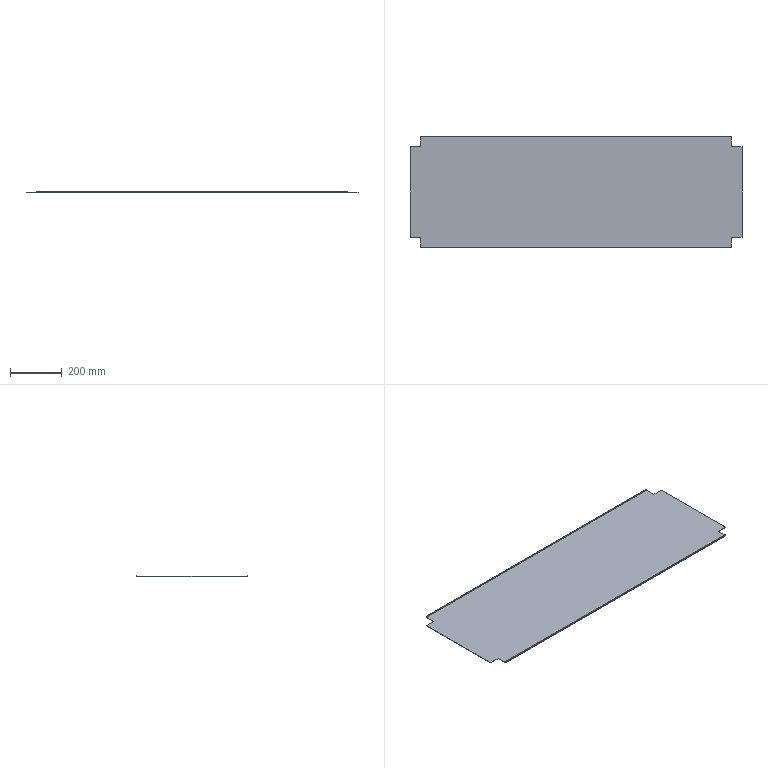Part | SolidWorks | features Extrusion 1, ICE 1 | 1 solid | 18 faces | box 1280 x 430 x 6.5 mm | volume 834000 mm3 | plane 18
STEP:
#1=CARTESIAN_POINT('',(40.,40.,1.5));
#2=VERTEX_POINT('',#1);
#3=CARTESIAN_POINT('',(40.,1.5,1.5));
#4=VERTEX_POINT('',#3);
#5=CARTESIAN_POINT('',(40.,0.,1.5));
#6=DIRECTION('',(0.,-1.,0.));
#7=VECTOR('',#6,1000.);
#8=LINE('',#5,#7);
#9=EDGE_CURVE('',#2,#4,#8,.T.);
#10=ORIENTED_EDGE('',*,*,#9,.T.);
#11=CARTESIAN_POINT('',(1240.,1.5,1.5));
#12=VERTEX_POINT('',#11);
#13=CARTESIAN_POINT('',(40.,1.5,1.5));
#14=DIRECTION('',(-1.,0.,0.));
#15=VECTOR('',#14,1000.);
#16=LINE('',#13,#15);
#17=EDGE_CURVE('',#12,#4,#16,.T.);
#18=ORIENTED_EDGE('',*,*,#17,.F.);
#19=CARTESIAN_POINT('',(1240.,40.,1.5));
#20=VERTEX_POINT('',#19);
#21=CARTESIAN_POINT('',(1240.,0.,1.5));
#22=DIRECTION('',(0.,1.,0.));
#23=VECTOR('',#22,1000.);
#24=LINE('',#21,#23);
#25=EDGE_CURVE('',#12,#20,#24,.T.);
#26=ORIENTED_EDGE('',*,*,#25,.T.);
#27=CARTESIAN_POINT('',(1280.,40.,1.5));
#28=VERTEX_POINT('',#27);
#29=CARTESIAN_POINT('',(1280.,40.,1.5));
#30=DIRECTION('',(1.,0.,0.));
#31=VECTOR('',#30,1000.);
#32=LINE('',#29,#31);
#33=EDGE_CURVE('',#20,#28,#32,.T.);
#34=ORIENTED_EDGE('',*,*,#33,.T.);
#35=CARTESIAN_POINT('',(1280.,390.,1.5));
#36=VERTEX_POINT('',#35);
#37=CARTESIAN_POINT('',(1280.,40.,1.5));
#38=DIRECTION('',(0.,1.,0.));
#39=VECTOR('',#38,1000.);
#40=LINE('',#37,#39);
#41=EDGE_CURVE('',#28,#36,#40,.T.);
#42=ORIENTED_EDGE('',*,*,#41,.T.);
#43=CARTESIAN_POINT('',(1240.,390.,1.5));
#44=VERTEX_POINT('',#43);
#45=CARTESIAN_POINT('',(1280.,390.,1.5));
#46=DIRECTION('',(-1.,0.,0.));
#47=VECTOR('',#46,1000.);
#48=LINE('',#45,#47);
#49=EDGE_CURVE('',#36,#44,#48,.T.);
#50=ORIENTED_EDGE('',*,*,#49,.T.);
#51=CARTESIAN_POINT('',(1240.,428.5,1.5));
#52=VERTEX_POINT('',#51);
#53=CARTESIAN_POINT('',(1240.,430.,1.5));
#54=DIRECTION('',(0.,1.,0.));
#55=VECTOR('',#54,1000.);
#56=LINE('',#53,#55);
#57=EDGE_CURVE('',#44,#52,#56,.T.);
#58=ORIENTED_EDGE('',*,*,#57,.T.);
#59=CARTESIAN_POINT('',(40.,428.5,1.5));
#60=VERTEX_POINT('',#59);
#61=CARTESIAN_POINT('',(40.,428.5,1.5));
#62=DIRECTION('',(1.,0.,0.));
#63=VECTOR('',#62,1000.);
#64=LINE('',#61,#63);
#65=EDGE_CURVE('',#60,#52,#64,.T.);
#66=ORIENTED_EDGE('',*,*,#65,.F.);
#67=CARTESIAN_POINT('',(40.,390.,1.5));
#68=VERTEX_POINT('',#67);
#69=CARTESIAN_POINT('',(40.,430.,1.5));
#70=DIRECTION('',(0.,-1.,0.));
#71=VECTOR('',#70,1000.);
#72=LINE('',#69,#71);
#73=EDGE_CURVE('',#60,#68,#72,.T.);
#74=ORIENTED_EDGE('',*,*,#73,.T.);
#75=CARTESIAN_POINT('',(0.,390.,1.5));
#76=VERTEX_POINT('',#75);
#77=CARTESIAN_POINT('',(0.,390.,1.5));
#78=DIRECTION('',(-1.,0.,0.));
#79=VECTOR('',#78,1000.);
#80=LINE('',#77,#79);
#81=EDGE_CURVE('',#68,#76,#80,.T.);
#82=ORIENTED_EDGE('',*,*,#81,.T.);
#83=CARTESIAN_POINT('',(0.,40.,1.5));
#84=VERTEX_POINT('',#83);
#85=CARTESIAN_POINT('',(0.,40.,1.5));
#86=DIRECTION('',(0.,-1.,0.));
#87=VECTOR('',#86,1000.);
#88=LINE('',#85,#87);
#89=EDGE_CURVE('',#76,#84,#88,.T.);
#90=ORIENTED_EDGE('',*,*,#89,.T.);
#91=CARTESIAN_POINT('',(0.,40.,1.5));
#92=DIRECTION('',(1.,0.,0.));
#93=VECTOR('',#92,1000.);
#94=LINE('',#91,#93);
#95=EDGE_CURVE('',#84,#2,#94,.T.);
#96=ORIENTED_EDGE('',*,*,#95,.T.);
#97=EDGE_LOOP('',(#10,#18,#26,#34,#42,#50,#58,#66,#74,#82,#90,#96));
#98=FACE_OUTER_BOUND('',#97,.T.);
#99=CARTESIAN_POINT('',(0.,0.,1.5));
#100=DIRECTION('',(0.,0.,1.));
#101=DIRECTION('',(1.,0.,0.));
#102=AXIS2_PLACEMENT_3D('',#99,#100,#101);
#103=PLANE('',#102);
#104=ADVANCED_FACE('',(#98),#103,.T.);
#105=CARTESIAN_POINT('',(40.,430.,0.));
#106=VERTEX_POINT('',#105);
#107=CARTESIAN_POINT('',(40.,390.,0.));
#108=VERTEX_POINT('',#107);
#109=CARTESIAN_POINT('',(40.,430.,0.));
#110=DIRECTION('',(0.,-1.,0.));
#111=VECTOR('',#110,1000.);
#112=LINE('',#109,#111);
#113=EDGE_CURVE('',#106,#108,#112,.T.);
#114=ORIENTED_EDGE('',*,*,#113,.T.);
#115=CARTESIAN_POINT('',(40.,390.,1.5));
#116=DIRECTION('',(0.,0.,-1.));
#117=VECTOR('',#116,1000.);
#118=LINE('',#115,#117);
#119=EDGE_CURVE('',#68,#108,#118,.T.);
#120=ORIENTED_EDGE('',*,*,#119,.F.);
#121=ORIENTED_EDGE('',*,*,#73,.F.);
#122=CARTESIAN_POINT('',(40.,428.5,6.5));
#123=VERTEX_POINT('',#122);
#124=CARTESIAN_POINT('',(40.,428.5,6.5));
#125=DIRECTION('',(0.,0.,-1.));
#126=VECTOR('',#125,1000.);
#127=LINE('',#124,#126);
#128=EDGE_CURVE('',#123,#60,#127,.T.);
#129=ORIENTED_EDGE('',*,*,#128,.F.);
#130=CARTESIAN_POINT('',(40.,430.,6.5));
#131=VERTEX_POINT('',#130);
#132=CARTESIAN_POINT('',(40.,430.,6.5));
#133=DIRECTION('',(0.,-1.,0.));
#134=VECTOR('',#133,1000.);
#135=LINE('',#132,#134);
#136=EDGE_CURVE('',#131,#123,#135,.T.);
#137=ORIENTED_EDGE('',*,*,#136,.F.);
#138=CARTESIAN_POINT('',(40.,430.,1.5));
#139=DIRECTION('',(0.,0.,-1.));
#140=VECTOR('',#139,1000.);
#141=LINE('',#138,#140);
#142=EDGE_CURVE('',#131,#106,#141,.T.);
#143=ORIENTED_EDGE('',*,*,#142,.T.);
#144=EDGE_LOOP('',(#114,#120,#121,#129,#137,#143));
#145=FACE_OUTER_BOUND('',#144,.T.);
#146=CARTESIAN_POINT('',(40.,430.,1.5));
#147=DIRECTION('',(1.,0.,0.));
#148=DIRECTION('',(0.,0.,-1.));
#149=AXIS2_PLACEMENT_3D('',#146,#147,#148);
#150=PLANE('',#149);
#151=ADVANCED_FACE('',(#145),#150,.F.);
#152=CARTESIAN_POINT('',(0.,390.,0.));
#153=VERTEX_POINT('',#152);
#154=CARTESIAN_POINT('',(0.,390.,0.));
#155=DIRECTION('',(-1.,0.,0.));
#156=VECTOR('',#155,1000.);
#157=LINE('',#154,#156);
#158=EDGE_CURVE('',#108,#153,#157,.T.);
#159=ORIENTED_EDGE('',*,*,#158,.T.);
#160=CARTESIAN_POINT('',(0.,390.,1.5));
#161=DIRECTION('',(0.,0.,-1.));
#162=VECTOR('',#161,1000.);
#163=LINE('',#160,#162);
#164=EDGE_CURVE('',#76,#153,#163,.T.);
#165=ORIENTED_EDGE('',*,*,#164,.F.);
#166=ORIENTED_EDGE('',*,*,#81,.F.);
#167=ORIENTED_EDGE('',*,*,#119,.T.);
#168=EDGE_LOOP('',(#159,#165,#166,#167));
#169=FACE_OUTER_BOUND('',#168,.T.);
#170=CARTESIAN_POINT('',(0.,390.,1.5));
#171=DIRECTION('',(0.,-1.,0.));
#172=DIRECTION('',(0.,0.,-1.));
#173=AXIS2_PLACEMENT_3D('',#170,#171,#172);
#174=PLANE('',#173);
#175=ADVANCED_FACE('',(#169),#174,.F.);
#176=CARTESIAN_POINT('',(0.,40.,0.));
#177=VERTEX_POINT('',#176);
#178=CARTESIAN_POINT('',(0.,40.,0.));
#179=DIRECTION('',(0.,-1.,0.));
#180=VECTOR('',#179,1000.);
#181=LINE('',#178,#180);
#182=EDGE_CURVE('',#153,#177,#181,.T.);
#183=ORIENTED_EDGE('',*,*,#182,.T.);
#184=CARTESIAN_POINT('',(0.,40.,1.5));
#185=DIRECTION('',(0.,0.,-1.));
#186=VECTOR('',#185,1000.);
#187=LINE('',#184,#186);
#188=EDGE_CURVE('',#84,#177,#187,.T.);
#189=ORIENTED_EDGE('',*,*,#188,.F.);
#190=ORIENTED_EDGE('',*,*,#89,.F.);
#191=ORIENTED_EDGE('',*,*,#164,.T.);
#192=EDGE_LOOP('',(#183,#189,#190,#191));
#193=FACE_OUTER_BOUND('',#192,.T.);
#194=CARTESIAN_POINT('',(0.,40.,1.5));
#195=DIRECTION('',(1.,0.,0.));
#196=DIRECTION('',(0.,0.,-1.));
#197=AXIS2_PLACEMENT_3D('',#194,#195,#196);
#198=PLANE('',#197);
#199=ADVANCED_FACE('',(#193),#198,.F.);
#200=CARTESIAN_POINT('',(40.,40.,0.));
#201=VERTEX_POINT('',#200);
#202=CARTESIAN_POINT('',(0.,40.,0.));
#203=DIRECTION('',(1.,0.,0.));
#204=VECTOR('',#203,1000.);
#205=LINE('',#202,#204);
#206=EDGE_CURVE('',#177,#201,#205,.T.);
#207=ORIENTED_EDGE('',*,*,#206,.T.);
#208=CARTESIAN_POINT('',(40.,40.,1.5));
#209=DIRECTION('',(0.,0.,-1.));
#210=VECTOR('',#209,1000.);
#211=LINE('',#208,#210);
#212=EDGE_CURVE('',#2,#201,#211,.T.);
#213=ORIENTED_EDGE('',*,*,#212,.F.);
#214=ORIENTED_EDGE('',*,*,#95,.F.);
#215=ORIENTED_EDGE('',*,*,#188,.T.);
#216=EDGE_LOOP('',(#207,#213,#214,#215));
#217=FACE_OUTER_BOUND('',#216,.T.);
#218=CARTESIAN_POINT('',(0.,40.,1.5));
#219=DIRECTION('',(0.,1.,0.));
#220=DIRECTION('',(0.,0.,1.));
#221=AXIS2_PLACEMENT_3D('',#218,#219,#220);
#222=PLANE('',#221);
#223=ADVANCED_FACE('',(#217),#222,.F.);
#224=CARTESIAN_POINT('',(40.,0.,0.));
#225=VERTEX_POINT('',#224);
#226=CARTESIAN_POINT('',(40.,0.,0.));
#227=DIRECTION('',(0.,-1.,0.));
#228=VECTOR('',#227,1000.);
#229=LINE('',#226,#228);
#230=EDGE_CURVE('',#201,#225,#229,.T.);
#231=ORIENTED_EDGE('',*,*,#230,.T.);
#232=CARTESIAN_POINT('',(40.,0.,6.5));
#233=VERTEX_POINT('',#232);
#234=CARTESIAN_POINT('',(40.,0.,1.5));
#235=DIRECTION('',(0.,0.,-1.));
#236=VECTOR('',#235,1000.);
#237=LINE('',#234,#236);
#238=EDGE_CURVE('',#233,#225,#237,.T.);
#239=ORIENTED_EDGE('',*,*,#238,.F.);
#240=CARTESIAN_POINT('',(40.,1.5,6.5));
#241=VERTEX_POINT('',#240);
#242=CARTESIAN_POINT('',(40.,0.,6.5));
#243=DIRECTION('',(0.,-1.,0.));
#244=VECTOR('',#243,1000.);
#245=LINE('',#242,#244);
#246=EDGE_CURVE('',#241,#233,#245,.T.);
#247=ORIENTED_EDGE('',*,*,#246,.F.);
#248=CARTESIAN_POINT('',(40.,1.5,6.5));
#249=DIRECTION('',(0.,0.,-1.));
#250=VECTOR('',#249,1000.);
#251=LINE('',#248,#250);
#252=EDGE_CURVE('',#241,#4,#251,.T.);
#253=ORIENTED_EDGE('',*,*,#252,.T.);
#254=ORIENTED_EDGE('',*,*,#9,.F.);
#255=ORIENTED_EDGE('',*,*,#212,.T.);
#256=EDGE_LOOP('',(#231,#239,#247,#253,#254,#255));
#257=FACE_OUTER_BOUND('',#256,.T.);
#258=CARTESIAN_POINT('',(40.,0.,1.5));
#259=DIRECTION('',(1.,0.,0.));
#260=DIRECTION('',(0.,0.,-1.));
#261=AXIS2_PLACEMENT_3D('',#258,#259,#260);
#262=PLANE('',#261);
#263=ADVANCED_FACE('',(#257),#262,.F.);
#264=CARTESIAN_POINT('',(1240.,0.,0.));
#265=VERTEX_POINT('',#264);
#266=CARTESIAN_POINT('',(40.,0.,0.));
#267=DIRECTION('',(1.,0.,0.));
#268=VECTOR('',#267,1000.);
#269=LINE('',#266,#268);
#270=EDGE_CURVE('',#225,#265,#269,.T.);
#271=ORIENTED_EDGE('',*,*,#270,.T.);
#272=CARTESIAN_POINT('',(1240.,0.,6.5));
#273=VERTEX_POINT('',#272);
#274=CARTESIAN_POINT('',(1240.,0.,1.5));
#275=DIRECTION('',(0.,0.,-1.));
#276=VECTOR('',#275,1000.);
#277=LINE('',#274,#276);
#278=EDGE_CURVE('',#273,#265,#277,.T.);
#279=ORIENTED_EDGE('',*,*,#278,.F.);
#280=CARTESIAN_POINT('',(40.,0.,6.5));
#281=DIRECTION('',(1.,0.,0.));
#282=VECTOR('',#281,1000.);
#283=LINE('',#280,#282);
#284=EDGE_CURVE('',#233,#273,#283,.T.);
#285=ORIENTED_EDGE('',*,*,#284,.F.);
#286=ORIENTED_EDGE('',*,*,#238,.T.);
#287=EDGE_LOOP('',(#271,#279,#285,#286));
#288=FACE_OUTER_BOUND('',#287,.T.);
#289=CARTESIAN_POINT('',(40.,0.,1.5));
#290=DIRECTION('',(0.,1.,0.));
#291=DIRECTION('',(0.,0.,1.));
#292=AXIS2_PLACEMENT_3D('',#289,#290,#291);
#293=PLANE('',#292);
#294=ADVANCED_FACE('',(#288),#293,.F.);
#295=CARTESIAN_POINT('',(1240.,40.,0.));
#296=VERTEX_POINT('',#295);
#297=CARTESIAN_POINT('',(1240.,0.,0.));
#298=DIRECTION('',(0.,1.,0.));
#299=VECTOR('',#298,1000.);
#300=LINE('',#297,#299);
#301=EDGE_CURVE('',#265,#296,#300,.T.);
#302=ORIENTED_EDGE('',*,*,#301,.T.);
#303=CARTESIAN_POINT('',(1240.,40.,1.5));
#304=DIRECTION('',(0.,0.,-1.));
#305=VECTOR('',#304,1000.);
#306=LINE('',#303,#305);
#307=EDGE_CURVE('',#20,#296,#306,.T.);
#308=ORIENTED_EDGE('',*,*,#307,.F.);
#309=ORIENTED_EDGE('',*,*,#25,.F.);
#310=CARTESIAN_POINT('',(1240.,1.5,6.5));
#311=VERTEX_POINT('',#310);
#312=CARTESIAN_POINT('',(1240.,1.5,6.5));
#313=DIRECTION('',(0.,0.,-1.));
#314=VECTOR('',#313,1000.);
#315=LINE('',#312,#314);
#316=EDGE_CURVE('',#311,#12,#315,.T.);
#317=ORIENTED_EDGE('',*,*,#316,.F.);
#318=CARTESIAN_POINT('',(1240.,0.,6.5));
#319=DIRECTION('',(0.,1.,0.));
#320=VECTOR('',#319,1000.);
#321=LINE('',#318,#320);
#322=EDGE_CURVE('',#273,#311,#321,.T.);
#323=ORIENTED_EDGE('',*,*,#322,.F.);
#324=ORIENTED_EDGE('',*,*,#278,.T.);
#325=EDGE_LOOP('',(#302,#308,#309,#317,#323,#324));
#326=FACE_OUTER_BOUND('',#325,.T.);
#327=CARTESIAN_POINT('',(1240.,0.,1.5));
#328=DIRECTION('',(-1.,0.,0.));
#329=DIRECTION('',(0.,0.,1.));
#330=AXIS2_PLACEMENT_3D('',#327,#328,#329);
#331=PLANE('',#330);
#332=ADVANCED_FACE('',(#326),#331,.F.);
#333=CARTESIAN_POINT('',(1280.,40.,0.));
#334=VERTEX_POINT('',#333);
#335=CARTESIAN_POINT('',(1280.,40.,0.));
#336=DIRECTION('',(1.,0.,0.));
#337=VECTOR('',#336,1000.);
#338=LINE('',#335,#337);
#339=EDGE_CURVE('',#296,#334,#338,.T.);
#340=ORIENTED_EDGE('',*,*,#339,.T.);
#341=CARTESIAN_POINT('',(1280.,40.,1.5));
#342=DIRECTION('',(0.,0.,-1.));
#343=VECTOR('',#342,1000.);
#344=LINE('',#341,#343);
#345=EDGE_CURVE('',#28,#334,#344,.T.);
#346=ORIENTED_EDGE('',*,*,#345,.F.);
#347=ORIENTED_EDGE('',*,*,#33,.F.);
#348=ORIENTED_EDGE('',*,*,#307,.T.);
#349=EDGE_LOOP('',(#340,#346,#347,#348));
#350=FACE_OUTER_BOUND('',#349,.T.);
#351=CARTESIAN_POINT('',(1280.,40.,1.5));
#352=DIRECTION('',(0.,1.,0.));
#353=DIRECTION('',(0.,0.,1.));
#354=AXIS2_PLACEMENT_3D('',#351,#352,#353);
#355=PLANE('',#354);
#356=ADVANCED_FACE('',(#350),#355,.F.);
#357=CARTESIAN_POINT('',(1280.,390.,0.));
#358=VERTEX_POINT('',#357);
#359=CARTESIAN_POINT('',(1280.,40.,0.));
#360=DIRECTION('',(0.,1.,0.));
#361=VECTOR('',#360,1000.);
#362=LINE('',#359,#361);
#363=EDGE_CURVE('',#334,#358,#362,.T.);
#364=ORIENTED_EDGE('',*,*,#363,.T.);
#365=CARTESIAN_POINT('',(1280.,390.,1.5));
#366=DIRECTION('',(0.,0.,-1.));
#367=VECTOR('',#366,1000.);
#368=LINE('',#365,#367);
#369=EDGE_CURVE('',#36,#358,#368,.T.);
#370=ORIENTED_EDGE('',*,*,#369,.F.);
#371=ORIENTED_EDGE('',*,*,#41,.F.);
#372=ORIENTED_EDGE('',*,*,#345,.T.);
#373=EDGE_LOOP('',(#364,#370,#371,#372));
#374=FACE_OUTER_BOUND('',#373,.T.);
#375=CARTESIAN_POINT('',(1280.,40.,1.5));
#376=DIRECTION('',(-1.,0.,0.));
#377=DIRECTION('',(0.,0.,1.));
#378=AXIS2_PLACEMENT_3D('',#375,#376,#377);
#379=PLANE('',#378);
#380=ADVANCED_FACE('',(#374),#379,.F.);
#381=CARTESIAN_POINT('',(1240.,390.,0.));
#382=VERTEX_POINT('',#381);
#383=CARTESIAN_POINT('',(1280.,390.,0.));
#384=DIRECTION('',(-1.,0.,0.));
#385=VECTOR('',#384,1000.);
#386=LINE('',#383,#385);
#387=EDGE_CURVE('',#358,#382,#386,.T.);
#388=ORIENTED_EDGE('',*,*,#387,.T.);
#389=CARTESIAN_POINT('',(1240.,390.,1.5));
#390=DIRECTION('',(0.,0.,-1.));
#391=VECTOR('',#390,1000.);
#392=LINE('',#389,#391);
#393=EDGE_CURVE('',#44,#382,#392,.T.);
#394=ORIENTED_EDGE('',*,*,#393,.F.);
#395=ORIENTED_EDGE('',*,*,#49,.F.);
#396=ORIENTED_EDGE('',*,*,#369,.T.);
#397=EDGE_LOOP('',(#388,#394,#395,#396));
#398=FACE_OUTER_BOUND('',#397,.T.);
#399=CARTESIAN_POINT('',(1280.,390.,1.5));
#400=DIRECTION('',(0.,-1.,0.));
#401=DIRECTION('',(0.,0.,-1.));
#402=AXIS2_PLACEMENT_3D('',#399,#400,#401);
#403=PLANE('',#402);
#404=ADVANCED_FACE('',(#398),#403,.F.);
#405=CARTESIAN_POINT('',(1240.,430.,0.));
#406=VERTEX_POINT('',#405);
#407=CARTESIAN_POINT('',(1240.,430.,0.));
#408=DIRECTION('',(0.,1.,0.));
#409=VECTOR('',#408,1000.);
#410=LINE('',#407,#409);
#411=EDGE_CURVE('',#382,#406,#410,.T.);
#412=ORIENTED_EDGE('',*,*,#411,.T.);
#413=CARTESIAN_POINT('',(1240.,430.,6.5));
#414=VERTEX_POINT('',#413);
#415=CARTESIAN_POINT('',(1240.,430.,1.5));
#416=DIRECTION('',(0.,0.,-1.));
#417=VECTOR('',#416,1000.);
#418=LINE('',#415,#417);
#419=EDGE_CURVE('',#414,#406,#418,.T.);
#420=ORIENTED_EDGE('',*,*,#419,.F.);
#421=CARTESIAN_POINT('',(1240.,428.5,6.5));
#422=VERTEX_POINT('',#421);
#423=CARTESIAN_POINT('',(1240.,430.,6.5));
#424=DIRECTION('',(0.,1.,0.));
#425=VECTOR('',#424,1000.);
#426=LINE('',#423,#425);
#427=EDGE_CURVE('',#422,#414,#426,.T.);
#428=ORIENTED_EDGE('',*,*,#427,.F.);
#429=CARTESIAN_POINT('',(1240.,428.5,6.5));
#430=DIRECTION('',(0.,0.,-1.));
#431=VECTOR('',#430,1000.);
#432=LINE('',#429,#431);
#433=EDGE_CURVE('',#422,#52,#432,.T.);
#434=ORIENTED_EDGE('',*,*,#433,.T.);
#435=ORIENTED_EDGE('',*,*,#57,.F.);
#436=ORIENTED_EDGE('',*,*,#393,.T.);
#437=EDGE_LOOP('',(#412,#420,#428,#434,#435,#436));
#438=FACE_OUTER_BOUND('',#437,.T.);
#439=CARTESIAN_POINT('',(1240.,430.,1.5));
#440=DIRECTION('',(-1.,0.,0.));
#441=DIRECTION('',(0.,0.,1.));
#442=AXIS2_PLACEMENT_3D('',#439,#440,#441);
#443=PLANE('',#442);
#444=ADVANCED_FACE('',(#438),#443,.F.);
#445=CARTESIAN_POINT('',(40.,430.,0.));
#446=DIRECTION('',(-1.,0.,0.));
#447=VECTOR('',#446,1000.);
#448=LINE('',#445,#447);
#449=EDGE_CURVE('',#406,#106,#448,.T.);
#450=ORIENTED_EDGE('',*,*,#449,.T.);
#451=ORIENTED_EDGE('',*,*,#142,.F.);
#452=CARTESIAN_POINT('',(40.,430.,6.5));
#453=DIRECTION('',(-1.,0.,0.));
#454=VECTOR('',#453,1000.);
#455=LINE('',#452,#454);
#456=EDGE_CURVE('',#414,#131,#455,.T.);
#457=ORIENTED_EDGE('',*,*,#456,.F.);
#458=ORIENTED_EDGE('',*,*,#419,.T.);
#459=EDGE_LOOP('',(#450,#451,#457,#458));
#460=FACE_OUTER_BOUND('',#459,.T.);
#461=CARTESIAN_POINT('',(40.,430.,1.5));
#462=DIRECTION('',(0.,-1.,0.));
#463=DIRECTION('',(1.,0.,0.));
#464=AXIS2_PLACEMENT_3D('',#461,#462,#463);
#465=PLANE('',#464);
#466=ADVANCED_FACE('',(#460),#465,.F.);
#467=ORIENTED_EDGE('',*,*,#113,.F.);
#468=ORIENTED_EDGE('',*,*,#449,.F.);
#469=ORIENTED_EDGE('',*,*,#411,.F.);
#470=ORIENTED_EDGE('',*,*,#387,.F.);
#471=ORIENTED_EDGE('',*,*,#363,.F.);
#472=ORIENTED_EDGE('',*,*,#339,.F.);
#473=ORIENTED_EDGE('',*,*,#301,.F.);
#474=ORIENTED_EDGE('',*,*,#270,.F.);
#475=ORIENTED_EDGE('',*,*,#230,.F.);
#476=ORIENTED_EDGE('',*,*,#206,.F.);
#477=ORIENTED_EDGE('',*,*,#182,.F.);
#478=ORIENTED_EDGE('',*,*,#158,.F.);
#479=EDGE_LOOP('',(#467,#468,#469,#470,#471,#472,#473,#474,#475,#476,#477,#478));
#480=FACE_OUTER_BOUND('',#479,.T.);
#481=CARTESIAN_POINT('',(0.,0.,0.));
#482=DIRECTION('',(0.,0.,1.));
#483=DIRECTION('',(1.,0.,0.));
#484=AXIS2_PLACEMENT_3D('',#481,#482,#483);
#485=PLANE('',#484);
#486=ADVANCED_FACE('',(#480),#485,.F.);
#487=ORIENTED_EDGE('',*,*,#65,.T.);
#488=ORIENTED_EDGE('',*,*,#433,.F.);
#489=CARTESIAN_POINT('',(40.,428.5,6.5));
#490=DIRECTION('',(1.,0.,0.));
#491=VECTOR('',#490,1000.);
#492=LINE('',#489,#491);
#493=EDGE_CURVE('',#123,#422,#492,.T.);
#494=ORIENTED_EDGE('',*,*,#493,.F.);
#495=ORIENTED_EDGE('',*,*,#128,.T.);
#496=EDGE_LOOP('',(#487,#488,#494,#495));
#497=FACE_OUTER_BOUND('',#496,.T.);
#498=CARTESIAN_POINT('',(40.,428.5,6.5));
#499=DIRECTION('',(0.,1.,0.));
#500=DIRECTION('',(0.,0.,1.));
#501=AXIS2_PLACEMENT_3D('',#498,#499,#500);
#502=PLANE('',#501);
#503=ADVANCED_FACE('',(#497),#502,.F.);
#504=ORIENTED_EDGE('',*,*,#136,.T.);
#505=ORIENTED_EDGE('',*,*,#493,.T.);
#506=ORIENTED_EDGE('',*,*,#427,.T.);
#507=ORIENTED_EDGE('',*,*,#456,.T.);
#508=EDGE_LOOP('',(#504,#505,#506,#507));
#509=FACE_OUTER_BOUND('',#508,.T.);
#510=CARTESIAN_POINT('',(0.,0.,6.5));
#511=DIRECTION('',(0.,0.,1.));
#512=DIRECTION('',(1.,0.,0.));
#513=AXIS2_PLACEMENT_3D('',#510,#511,#512);
#514=PLANE('',#513);
#515=ADVANCED_FACE('',(#509),#514,.T.);
#516=ORIENTED_EDGE('',*,*,#17,.T.);
#517=ORIENTED_EDGE('',*,*,#252,.F.);
#518=CARTESIAN_POINT('',(40.,1.5,6.5));
#519=DIRECTION('',(-1.,0.,0.));
#520=VECTOR('',#519,1000.);
#521=LINE('',#518,#520);
#522=EDGE_CURVE('',#311,#241,#521,.T.);
#523=ORIENTED_EDGE('',*,*,#522,.F.);
#524=ORIENTED_EDGE('',*,*,#316,.T.);
#525=EDGE_LOOP('',(#516,#517,#523,#524));
#526=FACE_OUTER_BOUND('',#525,.T.);
#527=CARTESIAN_POINT('',(40.,1.5,6.5));
#528=DIRECTION('',(0.,-1.,0.));
#529=DIRECTION('',(0.,0.,-1.));
#530=AXIS2_PLACEMENT_3D('',#527,#528,#529);
#531=PLANE('',#530);
#532=ADVANCED_FACE('',(#526),#531,.F.);
#533=ORIENTED_EDGE('',*,*,#246,.T.);
#534=ORIENTED_EDGE('',*,*,#284,.T.);
#535=ORIENTED_EDGE('',*,*,#322,.T.);
#536=ORIENTED_EDGE('',*,*,#522,.T.);
#537=EDGE_LOOP('',(#533,#534,#535,#536));
#538=FACE_OUTER_BOUND('',#537,.T.);
#539=CARTESIAN_POINT('',(0.,0.,6.5));
#540=DIRECTION('',(0.,0.,-1.));
#541=DIRECTION('',(-1.,0.,0.));
#542=AXIS2_PLACEMENT_3D('',#539,#540,#541);
#543=PLANE('',#542);
#544=ADVANCED_FACE('',(#538),#543,.F.);
#545=CLOSED_SHELL('',(#104,#151,#175,#199,#223,#263,#294,#332,#356,#380,#404,#444,#466,#486,#503,#515,#532,#544));
#546=MANIFOLD_SOLID_BREP('',#545);
#547=CARTESIAN_POINT('',(0.,0.,0.));
#548=DIRECTION('',(0.,0.,1.));
#549=DIRECTION('',(1.,0.,0.));
#550=AXIS2_PLACEMENT_3D('',#547,#548,#549);
#551=(LENGTH_UNIT()NAMED_UNIT(*)SI_UNIT(.MILLI.,.METRE.));
#552=UNCERTAINTY_MEASURE_WITH_UNIT(LENGTH_MEASURE(0.00001),#551,'','');
#553=(NAMED_UNIT(*)PLANE_ANGLE_UNIT()SI_UNIT($,.RADIAN.));
#554=(NAMED_UNIT(*)SI_UNIT($,.STERADIAN.)SOLID_ANGLE_UNIT());
#555=(GEOMETRIC_REPRESENTATION_CONTEXT(3)GLOBAL_UNCERTAINTY_ASSIGNED_CONTEXT((#552))GLOBAL_UNIT_ASSIGNED_CONTEXT((#551,#553,#554))REPRESENTATION_CONTEXT('',''));
#556=ADVANCED_BREP_SHAPE_REPRESENTATION('',(#546,#550),#555);